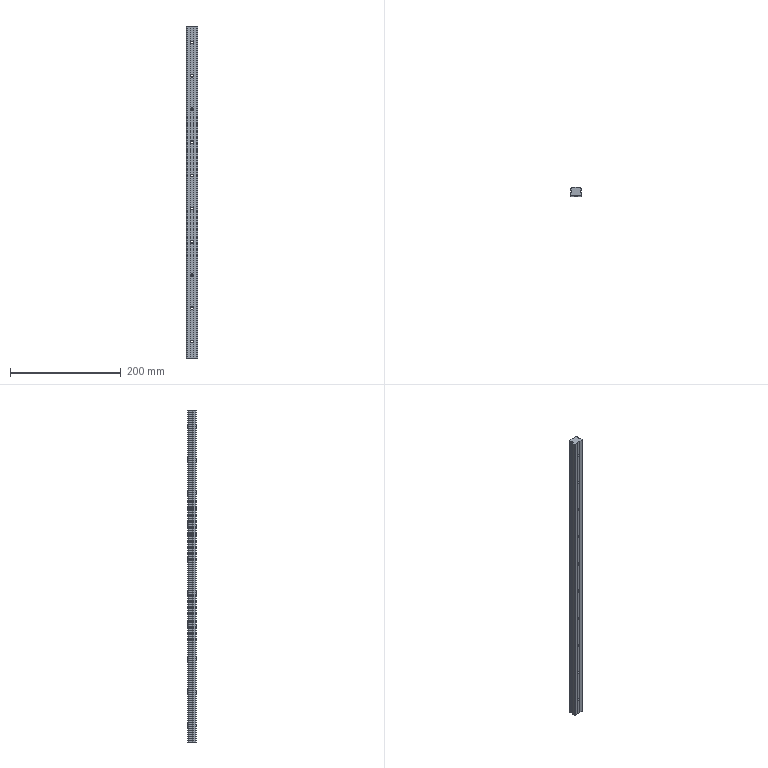Part | SolidWorks | features 3DProfileFeature 1, Extrusion 1, HoleWzd 1, LPattern 1 | 1 solid | 88 faces | box 20 x 15.5 x 600 mm | volume 162384 mm3 | cylinder 58 | plane 30 | commonest cylinder face diameters 4.5 x20 8 x20 1 x12 4.333 x4 2 x2